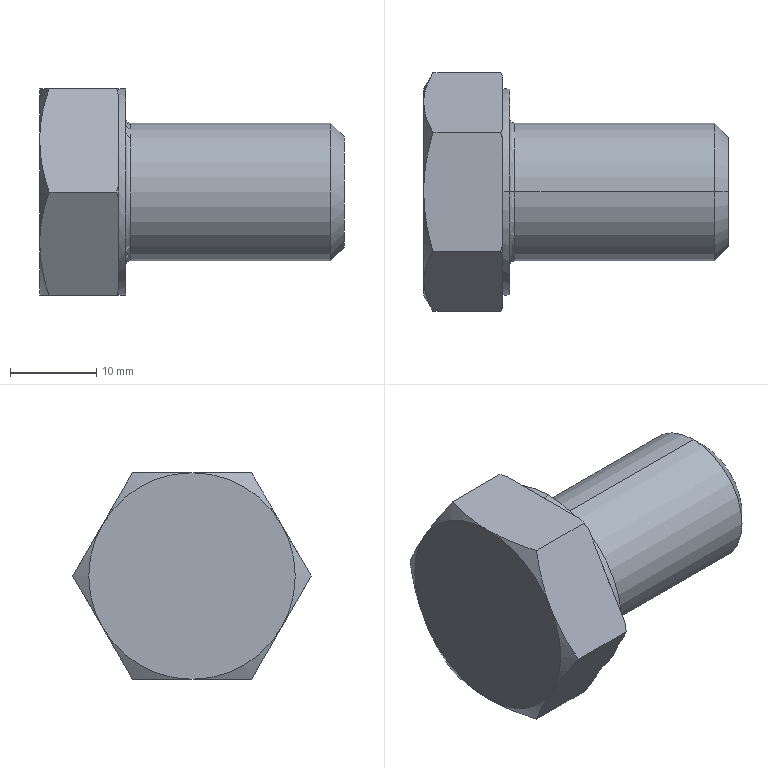Part | SolidWorks | features RevCut 4, Chamfer 1, Extrusion 1, Fillet 1, LPattern 1, Revolution 1 | 1 solid | 35 faces | box 35.4 x 27.713 x 24 mm | volume 9987 mm3 | plane 15 | cone 14 | cylinder 4 | torus 2 | commonest cylinder face diameters 16 x2 24 x2
STEP:
#1=CARTESIAN_POINT('',(10.6,0.,8.));
#2=VERTEX_POINT('',#1);
#3=CARTESIAN_POINT('',(10.6,0.,-8.));
#4=VERTEX_POINT('',#3);
#5=CARTESIAN_POINT('',(10.6,0.,0.));
#6=DIRECTION('',(1.,0.,0.));
#7=DIRECTION('',(0.,0.,-1.));
#8=AXIS2_PLACEMENT_3D('',#5,#6,#7);
#9=CIRCLE('',#8,8.);
#10=EDGE_CURVE('',#2,#4,#9,.T.);
#11=ORIENTED_EDGE('',*,*,#10,.F.);
#12=CARTESIAN_POINT('',(10.,0.,8.6));
#13=VERTEX_POINT('',#12);
#14=CARTESIAN_POINT('',(10.6,0.,8.6));
#15=DIRECTION('',(0.,1.,0.));
#16=DIRECTION('',(0.,0.,1.));
#17=AXIS2_PLACEMENT_3D('',#14,#15,#16);
#18=CIRCLE('',#17,0.6);
#19=EDGE_CURVE('',#2,#13,#18,.T.);
#20=ORIENTED_EDGE('',*,*,#19,.T.);
#21=CARTESIAN_POINT('',(10.,0.,-8.6));
#22=VERTEX_POINT('',#21);
#23=CARTESIAN_POINT('',(10.,0.,0.));
#24=DIRECTION('',(-1.,0.,0.));
#25=DIRECTION('',(0.,0.,-1.));
#26=AXIS2_PLACEMENT_3D('',#23,#24,#25);
#27=CIRCLE('',#26,8.6);
#28=EDGE_CURVE('',#22,#13,#27,.T.);
#29=ORIENTED_EDGE('',*,*,#28,.F.);
#30=CARTESIAN_POINT('',(10.6,0.,-8.6));
#31=DIRECTION('',(0.,-1.,0.));
#32=DIRECTION('',(0.,0.,-1.));
#33=AXIS2_PLACEMENT_3D('',#30,#31,#32);
#34=CIRCLE('',#33,0.6);
#35=EDGE_CURVE('',#4,#22,#34,.T.);
#36=ORIENTED_EDGE('',*,*,#35,.F.);
#37=EDGE_LOOP('',(#11,#20,#29,#36));
#38=FACE_OUTER_BOUND('',#37,.T.);
#39=CARTESIAN_POINT('',(10.6,0.,0.));
#40=DIRECTION('',(1.,0.,0.));
#41=DIRECTION('',(0.,0.,-1.));
#42=AXIS2_PLACEMENT_3D('',#39,#40,#41);
#43=TOROIDAL_SURFACE('',#42,8.6,0.6);
#44=ADVANCED_FACE('',(#38),#43,.F.);
#45=CARTESIAN_POINT('',(35.4,0.,-6.4));
#46=VERTEX_POINT('',#45);
#47=CARTESIAN_POINT('',(35.4,0.,6.4));
#48=VERTEX_POINT('',#47);
#49=CARTESIAN_POINT('',(35.4,0.,0.));
#50=DIRECTION('',(1.,0.,0.));
#51=DIRECTION('',(0.,0.,1.));
#52=AXIS2_PLACEMENT_3D('',#49,#50,#51);
#53=CIRCLE('',#52,6.4);
#54=EDGE_CURVE('',#46,#48,#53,.T.);
#55=ORIENTED_EDGE('',*,*,#54,.F.);
#56=CARTESIAN_POINT('',(33.8,0.,-8.));
#57=VERTEX_POINT('',#56);
#58=CARTESIAN_POINT('',(33.8,0.,-8.));
#59=DIRECTION('',(-0.7071,0.,-0.7071));
#60=VECTOR('',#59,1000.);
#61=LINE('',#58,#60);
#62=EDGE_CURVE('',#46,#57,#61,.T.);
#63=ORIENTED_EDGE('',*,*,#62,.T.);
#64=CARTESIAN_POINT('',(33.8,0.,8.));
#65=VERTEX_POINT('',#64);
#66=CARTESIAN_POINT('',(33.8,0.,0.));
#67=DIRECTION('',(-1.,0.,0.));
#68=DIRECTION('',(0.,0.,1.));
#69=AXIS2_PLACEMENT_3D('',#66,#67,#68);
#70=CIRCLE('',#69,8.);
#71=EDGE_CURVE('',#65,#57,#70,.T.);
#72=ORIENTED_EDGE('',*,*,#71,.F.);
#73=CARTESIAN_POINT('',(33.8,0.,8.));
#74=DIRECTION('',(-0.7071,0.,0.7071));
#75=VECTOR('',#74,1000.);
#76=LINE('',#73,#75);
#77=EDGE_CURVE('',#48,#65,#76,.T.);
#78=ORIENTED_EDGE('',*,*,#77,.F.);
#79=EDGE_LOOP('',(#55,#63,#72,#78));
#80=FACE_OUTER_BOUND('',#79,.T.);
#81=CARTESIAN_POINT('',(33.8,0.,0.));
#82=DIRECTION('',(-1.,0.,0.));
#83=DIRECTION('',(0.,0.,1.));
#84=AXIS2_PLACEMENT_3D('',#81,#82,#83);
#85=CONICAL_SURFACE('',#84,8.,0.7854);
#86=ADVANCED_FACE('',(#80),#85,.T.);
#87=ORIENTED_EDGE('',*,*,#71,.T.);
#88=CARTESIAN_POINT('',(0.,0.,-8.));
#89=DIRECTION('',(-1.,0.,0.));
#90=VECTOR('',#89,1000.);
#91=LINE('',#88,#90);
#92=EDGE_CURVE('',#57,#4,#91,.T.);
#93=ORIENTED_EDGE('',*,*,#92,.T.);
#94=CARTESIAN_POINT('',(10.6,0.,0.));
#95=DIRECTION('',(1.,0.,0.));
#96=DIRECTION('',(0.,0.,-1.));
#97=AXIS2_PLACEMENT_3D('',#94,#95,#96);
#98=CIRCLE('',#97,8.);
#99=EDGE_CURVE('',#4,#2,#98,.T.);
#100=ORIENTED_EDGE('',*,*,#99,.T.);
#101=CARTESIAN_POINT('',(0.,0.,8.));
#102=DIRECTION('',(-1.,0.,0.));
#103=VECTOR('',#102,1000.);
#104=LINE('',#101,#103);
#105=EDGE_CURVE('',#65,#2,#104,.T.);
#106=ORIENTED_EDGE('',*,*,#105,.F.);
#107=EDGE_LOOP('',(#87,#93,#100,#106));
#108=FACE_OUTER_BOUND('',#107,.T.);
#109=CARTESIAN_POINT('',(0.,0.,0.));
#110=DIRECTION('',(-1.,0.,0.));
#111=DIRECTION('',(0.,0.,1.));
#112=AXIS2_PLACEMENT_3D('',#109,#110,#111);
#113=CYLINDRICAL_SURFACE('',#112,8.);
#114=ADVANCED_FACE('',(#108),#113,.T.);
#115=CARTESIAN_POINT('',(10.,0.,-12.));
#116=VERTEX_POINT('',#115);
#117=CARTESIAN_POINT('',(10.,0.,12.));
#118=VERTEX_POINT('',#117);
#119=CARTESIAN_POINT('',(10.,0.,0.));
#120=DIRECTION('',(1.,0.,0.));
#121=DIRECTION('',(0.,0.,-1.));
#122=AXIS2_PLACEMENT_3D('',#119,#120,#121);
#123=CIRCLE('',#122,12.);
#124=EDGE_CURVE('',#116,#118,#123,.T.);
#125=ORIENTED_EDGE('',*,*,#124,.F.);
#126=CARTESIAN_POINT('',(9.2,0.,-12.));
#127=VERTEX_POINT('',#126);
#128=CARTESIAN_POINT('',(0.,0.,-12.));
#129=DIRECTION('',(-1.,0.,0.));
#130=VECTOR('',#129,1000.);
#131=LINE('',#128,#130);
#132=EDGE_CURVE('',#116,#127,#131,.T.);
#133=ORIENTED_EDGE('',*,*,#132,.T.);
#134=CARTESIAN_POINT('',(9.2,10.392,-6.));
#135=VERTEX_POINT('',#134);
#136=CARTESIAN_POINT('',(9.2,0.,0.));
#137=DIRECTION('',(-1.,0.,0.));
#138=DIRECTION('',(0.,0.,1.));
#139=AXIS2_PLACEMENT_3D('',#136,#137,#138);
#140=CIRCLE('',#139,12.);
#141=EDGE_CURVE('',#135,#127,#140,.T.);
#142=ORIENTED_EDGE('',*,*,#141,.F.);
#143=CARTESIAN_POINT('',(9.2,10.392,6.));
#144=VERTEX_POINT('',#143);
#145=CARTESIAN_POINT('',(9.2,0.,0.));
#146=DIRECTION('',(-1.,0.,0.));
#147=DIRECTION('',(0.,0.,1.));
#148=AXIS2_PLACEMENT_3D('',#145,#146,#147);
#149=CIRCLE('',#148,12.);
#150=EDGE_CURVE('',#144,#135,#149,.T.);
#151=ORIENTED_EDGE('',*,*,#150,.F.);
#152=CARTESIAN_POINT('',(9.2,0.,12.));
#153=VERTEX_POINT('',#152);
#154=CARTESIAN_POINT('',(9.2,0.,0.));
#155=DIRECTION('',(-1.,0.,0.));
#156=DIRECTION('',(0.,0.,1.));
#157=AXIS2_PLACEMENT_3D('',#154,#155,#156);
#158=CIRCLE('',#157,12.);
#159=EDGE_CURVE('',#153,#144,#158,.T.);
#160=ORIENTED_EDGE('',*,*,#159,.F.);
#161=CARTESIAN_POINT('',(0.,0.,12.));
#162=DIRECTION('',(-1.,0.,0.));
#163=VECTOR('',#162,1000.);
#164=LINE('',#161,#163);
#165=EDGE_CURVE('',#118,#153,#164,.T.);
#166=ORIENTED_EDGE('',*,*,#165,.F.);
#167=EDGE_LOOP('',(#125,#133,#142,#151,#160,#166));
#168=FACE_OUTER_BOUND('',#167,.T.);
#169=CARTESIAN_POINT('',(0.,0.,0.));
#170=DIRECTION('',(-1.,0.,0.));
#171=DIRECTION('',(0.,0.,1.));
#172=AXIS2_PLACEMENT_3D('',#169,#170,#171);
#173=CYLINDRICAL_SURFACE('',#172,12.);
#174=ADVANCED_FACE('',(#168),#173,.T.);
#175=CARTESIAN_POINT('',(9.2,7.427,-11.136));
#176=VERTEX_POINT('',#175);
#177=CARTESIAN_POINT('',(9.2,6.928,-12.));
#178=DIRECTION('',(0.,0.5,0.866));
#179=VECTOR('',#178,1000.);
#180=LINE('',#177,#179);
#181=EDGE_CURVE('',#176,#135,#180,.T.);
#182=ORIENTED_EDGE('',*,*,#181,.F.);
#183=CARTESIAN_POINT('',(8.928,6.928,-12.));
#184=VERTEX_POINT('',#183);
#185=CARTESIAN_POINT('',(8.928,6.928,-12.));
#186=CARTESIAN_POINT('',(9.024,7.094,-11.713));
#187=CARTESIAN_POINT('',(9.115,7.26,-11.425));
#188=CARTESIAN_POINT('',(9.2,7.427,-11.136));
#189=B_SPLINE_CURVE_WITH_KNOTS('',3,(#185,#186,#187,#188),.UNSPECIFIED.,.F.,.F.,(4,4),(0.000000238,0.001026),.UNSPECIFIED.);
#190=EDGE_CURVE('',#184,#176,#189,.T.);
#191=ORIENTED_EDGE('',*,*,#190,.F.);
#192=CARTESIAN_POINT('',(1.072,6.928,-12.));
#193=VERTEX_POINT('',#192);
#194=CARTESIAN_POINT('',(10.,6.928,-12.));
#195=DIRECTION('',(-1.,0.,0.));
#196=VECTOR('',#195,1000.);
#197=LINE('',#194,#196);
#198=EDGE_CURVE('',#184,#193,#197,.T.);
#199=ORIENTED_EDGE('',*,*,#198,.T.);
#200=CARTESIAN_POINT('',(0.,10.392,-6.));
#201=VERTEX_POINT('',#200);
#202=CARTESIAN_POINT('',(0.,10.392,-6.));
#203=CARTESIAN_POINT('',(0.,10.098,-6.509));
#204=CARTESIAN_POINT('',(0.02533,9.803,-7.021));
#205=CARTESIAN_POINT('',(0.1234,9.219,-8.033));
#206=CARTESIAN_POINT('',(0.196,8.929,-8.535));
#207=CARTESIAN_POINT('',(0.476,8.063,-10.034));
#208=CARTESIAN_POINT('',(0.7454,7.493,-11.021));
#209=CARTESIAN_POINT('',(1.072,6.928,-12.));
#210=B_SPLINE_CURVE_WITH_KNOTS('',3,(#202,#203,#204,#205,#206,#207,#208,#209),.UNSPECIFIED.,.F.,.F.,(4,2,2,4),(0.00701,0.008756,0.0105,0.01399),.UNSPECIFIED.);
#211=EDGE_CURVE('',#201,#193,#210,.T.);
#212=ORIENTED_EDGE('',*,*,#211,.F.);
#213=CARTESIAN_POINT('',(1.072,13.856,0.));
#214=VERTEX_POINT('',#213);
#215=CARTESIAN_POINT('',(1.072,13.856,0.));
#216=CARTESIAN_POINT('',(0.7446,13.29,-0.9815));
#217=CARTESIAN_POINT('',(0.4751,12.719,-1.97));
#218=CARTESIAN_POINT('',(0.1021,11.565,-3.968));
#219=CARTESIAN_POINT('',(0.,10.982,-4.978));
#220=CARTESIAN_POINT('',(0.,10.392,-6.));
#221=B_SPLINE_CURVE_WITH_KNOTS('',3,(#215,#216,#217,#218,#219,#220),.UNSPECIFIED.,.F.,.F.,(4,2,4),(0.000000238,0.003505,0.00701),.UNSPECIFIED.);
#222=EDGE_CURVE('',#214,#201,#221,.T.);
#223=ORIENTED_EDGE('',*,*,#222,.F.);
#224=CARTESIAN_POINT('',(8.928,13.856,0.));
#225=VERTEX_POINT('',#224);
#226=CARTESIAN_POINT('',(10.,13.856,0.));
#227=DIRECTION('',(-1.,0.,0.));
#228=VECTOR('',#227,1000.);
#229=LINE('',#226,#228);
#230=EDGE_CURVE('',#225,#214,#229,.T.);
#231=ORIENTED_EDGE('',*,*,#230,.F.);
#232=CARTESIAN_POINT('',(9.2,13.358,-0.8637));
#233=VERTEX_POINT('',#232);
#234=CARTESIAN_POINT('',(9.2,13.358,-0.8637));
#235=CARTESIAN_POINT('',(9.115,13.524,-0.575));
#236=CARTESIAN_POINT('',(9.024,13.691,-0.2872));
#237=CARTESIAN_POINT('',(8.928,13.856,0.));
#238=B_SPLINE_CURVE_WITH_KNOTS('',3,(#234,#235,#236,#237),.UNSPECIFIED.,.F.,.F.,(4,4),(0.01297,0.01399),.UNSPECIFIED.);
#239=EDGE_CURVE('',#233,#225,#238,.T.);
#240=ORIENTED_EDGE('',*,*,#239,.F.);
#241=CARTESIAN_POINT('',(9.2,6.928,-12.));
#242=DIRECTION('',(0.,0.5,0.866));
#243=VECTOR('',#242,1000.);
#244=LINE('',#241,#243);
#245=EDGE_CURVE('',#135,#233,#244,.T.);
#246=ORIENTED_EDGE('',*,*,#245,.F.);
#247=EDGE_LOOP('',(#182,#191,#199,#212,#223,#231,#240,#246));
#248=FACE_OUTER_BOUND('',#247,.T.);
#249=CARTESIAN_POINT('',(10.,6.928,-12.));
#250=DIRECTION('',(0.,-0.866,0.5));
#251=DIRECTION('',(0.,-0.5,-0.866));
#252=AXIS2_PLACEMENT_3D('',#249,#250,#251);
#253=PLANE('',#252);
#254=ADVANCED_FACE('',(#248),#253,.F.);
#255=CARTESIAN_POINT('',(9.2,13.358,0.8637));
#256=VERTEX_POINT('',#255);
#257=CARTESIAN_POINT('',(9.2,13.856,0.));
#258=DIRECTION('',(0.,-0.5,0.866));
#259=VECTOR('',#258,1000.);
#260=LINE('',#257,#259);
#261=EDGE_CURVE('',#256,#144,#260,.T.);
#262=ORIENTED_EDGE('',*,*,#261,.F.);
#263=CARTESIAN_POINT('',(8.928,13.856,0.));
#264=CARTESIAN_POINT('',(9.024,13.691,0.2873));
#265=CARTESIAN_POINT('',(9.115,13.524,0.5751));
#266=CARTESIAN_POINT('',(9.2,13.358,0.8637));
#267=B_SPLINE_CURVE_WITH_KNOTS('',3,(#263,#264,#265,#266),.UNSPECIFIED.,.F.,.F.,(4,4),(0.000000238,0.001026),.UNSPECIFIED.);
#268=EDGE_CURVE('',#225,#256,#267,.T.);
#269=ORIENTED_EDGE('',*,*,#268,.F.);
#270=ORIENTED_EDGE('',*,*,#230,.T.);
#271=CARTESIAN_POINT('',(0.,10.392,6.));
#272=VERTEX_POINT('',#271);
#273=CARTESIAN_POINT('',(0.,10.392,6.));
#274=CARTESIAN_POINT('',(0.,10.686,5.491));
#275=CARTESIAN_POINT('',(0.02533,10.982,4.979));
#276=CARTESIAN_POINT('',(0.1234,11.566,3.967));
#277=CARTESIAN_POINT('',(0.196,11.856,3.465));
#278=CARTESIAN_POINT('',(0.476,12.721,1.966));
#279=CARTESIAN_POINT('',(0.7454,13.291,0.9791));
#280=CARTESIAN_POINT('',(1.072,13.856,0.));
#281=B_SPLINE_CURVE_WITH_KNOTS('',3,(#273,#274,#275,#276,#277,#278,#279,#280),.UNSPECIFIED.,.F.,.F.,(4,2,2,4),(0.00701,0.008756,0.0105,0.01399),.UNSPECIFIED.);
#282=EDGE_CURVE('',#272,#214,#281,.T.);
#283=ORIENTED_EDGE('',*,*,#282,.F.);
#284=CARTESIAN_POINT('',(1.072,6.928,12.));
#285=VERTEX_POINT('',#284);
#286=CARTESIAN_POINT('',(1.072,6.928,12.));
#287=CARTESIAN_POINT('',(0.7446,7.495,11.018));
#288=CARTESIAN_POINT('',(0.4751,8.066,10.03));
#289=CARTESIAN_POINT('',(0.1021,9.219,8.032));
#290=CARTESIAN_POINT('',(0.,9.802,7.022));
#291=CARTESIAN_POINT('',(0.,10.392,6.));
#292=B_SPLINE_CURVE_WITH_KNOTS('',3,(#286,#287,#288,#289,#290,#291),.UNSPECIFIED.,.F.,.F.,(4,2,4),(0.000000238,0.003505,0.00701),.UNSPECIFIED.);
#293=EDGE_CURVE('',#285,#272,#292,.T.);
#294=ORIENTED_EDGE('',*,*,#293,.F.);
#295=CARTESIAN_POINT('',(8.928,6.928,12.));
#296=VERTEX_POINT('',#295);
#297=CARTESIAN_POINT('',(10.,6.928,12.));
#298=DIRECTION('',(-1.,0.,0.));
#299=VECTOR('',#298,1000.);
#300=LINE('',#297,#299);
#301=EDGE_CURVE('',#296,#285,#300,.T.);
#302=ORIENTED_EDGE('',*,*,#301,.F.);
#303=CARTESIAN_POINT('',(9.2,7.427,11.136));
#304=VERTEX_POINT('',#303);
#305=CARTESIAN_POINT('',(9.2,7.427,11.136));
#306=CARTESIAN_POINT('',(9.115,7.26,11.425));
#307=CARTESIAN_POINT('',(9.024,7.094,11.713));
#308=CARTESIAN_POINT('',(8.928,6.928,12.));
#309=B_SPLINE_CURVE_WITH_KNOTS('',3,(#305,#306,#307,#308),.UNSPECIFIED.,.F.,.F.,(4,4),(0.01297,0.01399),.UNSPECIFIED.);
#310=EDGE_CURVE('',#304,#296,#309,.T.);
#311=ORIENTED_EDGE('',*,*,#310,.F.);
#312=CARTESIAN_POINT('',(9.2,13.856,0.));
#313=DIRECTION('',(0.,-0.5,0.866));
#314=VECTOR('',#313,1000.);
#315=LINE('',#312,#314);
#316=EDGE_CURVE('',#144,#304,#315,.T.);
#317=ORIENTED_EDGE('',*,*,#316,.F.);
#318=EDGE_LOOP('',(#262,#269,#270,#283,#294,#302,#311,#317));
#319=FACE_OUTER_BOUND('',#318,.T.);
#320=CARTESIAN_POINT('',(10.,13.856,0.));
#321=DIRECTION('',(0.,-0.866,-0.5));
#322=DIRECTION('',(0.,0.5,-0.866));
#323=AXIS2_PLACEMENT_3D('',#320,#321,#322);
#324=PLANE('',#323);
#325=ADVANCED_FACE('',(#319),#324,.F.);
#326=CARTESIAN_POINT('',(9.2,5.931,12.));
#327=VERTEX_POINT('',#326);
#328=CARTESIAN_POINT('',(9.2,6.928,12.));
#329=DIRECTION('',(0.,-1.,0.));
#330=VECTOR('',#329,1000.);
#331=LINE('',#328,#330);
#332=EDGE_CURVE('',#327,#153,#331,.T.);
#333=ORIENTED_EDGE('',*,*,#332,.F.);
#334=CARTESIAN_POINT('',(8.928,6.928,12.));
#335=CARTESIAN_POINT('',(9.024,6.597,12.));
#336=CARTESIAN_POINT('',(9.115,6.265,12.));
#337=CARTESIAN_POINT('',(9.2,5.931,12.));
#338=B_SPLINE_CURVE_WITH_KNOTS('',3,(#334,#335,#336,#337),.UNSPECIFIED.,.F.,.F.,(4,4),(0.03236,0.0334),.UNSPECIFIED.);
#339=EDGE_CURVE('',#296,#327,#338,.T.);
#340=ORIENTED_EDGE('',*,*,#339,.F.);
#341=ORIENTED_EDGE('',*,*,#301,.T.);
#342=CARTESIAN_POINT('',(0.,0.,12.));
#343=VERTEX_POINT('',#342);
#344=CARTESIAN_POINT('',(0.,0.,12.));
#345=CARTESIAN_POINT('',(0.,0.5865,12.));
#346=CARTESIAN_POINT('',(0.02506,1.176,12.));
#347=CARTESIAN_POINT('',(0.1242,2.355,12.));
#348=CARTESIAN_POINT('',(0.1975,2.939,12.));
#349=CARTESIAN_POINT('',(0.4791,4.673,12.));
#350=CARTESIAN_POINT('',(0.7483,5.808,12.));
#351=CARTESIAN_POINT('',(1.072,6.928,12.));
#352=B_SPLINE_CURVE_WITH_KNOTS('',3,(#344,#345,#346,#347,#348,#349,#350,#351),.UNSPECIFIED.,.F.,.F.,(4,2,2,4),(0.01982,0.02158,0.02333,0.02684),.UNSPECIFIED.);
#353=EDGE_CURVE('',#343,#285,#352,.T.);
#354=ORIENTED_EDGE('',*,*,#353,.F.);
#355=CARTESIAN_POINT('',(1.072,-6.928,12.));
#356=VERTEX_POINT('',#355);
#357=CARTESIAN_POINT('',(1.072,-6.928,12.));
#358=CARTESIAN_POINT('',(0.7461,-5.8,12.));
#359=CARTESIAN_POINT('',(0.4736,-4.647,12.));
#360=CARTESIAN_POINT('',(0.1008,-2.335,12.));
#361=CARTESIAN_POINT('',(0.,-1.172,12.));
#362=CARTESIAN_POINT('',(0.,0.,12.));
#363=B_SPLINE_CURVE_WITH_KNOTS('',3,(#357,#358,#359,#360,#361,#362),.UNSPECIFIED.,.F.,.F.,(4,2,4),(0.01281,0.01632,0.01982),.UNSPECIFIED.);
#364=EDGE_CURVE('',#356,#343,#363,.T.);
#365=ORIENTED_EDGE('',*,*,#364,.F.);
#366=CARTESIAN_POINT('',(8.928,-6.928,12.));
#367=VERTEX_POINT('',#366);
#368=CARTESIAN_POINT('',(10.,-6.928,12.));
#369=DIRECTION('',(-1.,0.,0.));
#370=VECTOR('',#369,1000.);
#371=LINE('',#368,#370);
#372=EDGE_CURVE('',#367,#356,#371,.T.);
#373=ORIENTED_EDGE('',*,*,#372,.F.);
#374=CARTESIAN_POINT('',(9.2,-5.931,12.));
#375=VERTEX_POINT('',#374);
#376=CARTESIAN_POINT('',(9.2,-5.931,12.));
#377=CARTESIAN_POINT('',(9.114,-6.265,12.));
#378=CARTESIAN_POINT('',(9.024,-6.598,12.));
#379=CARTESIAN_POINT('',(8.928,-6.928,12.));
#380=B_SPLINE_CURVE_WITH_KNOTS('',3,(#376,#377,#378,#379),.UNSPECIFIED.,.F.,.F.,(4,4),(0.04537,0.0464),.UNSPECIFIED.);
#381=EDGE_CURVE('',#375,#367,#380,.T.);
#382=ORIENTED_EDGE('',*,*,#381,.F.);
#383=CARTESIAN_POINT('',(9.2,6.928,12.));
#384=DIRECTION('',(0.,-1.,0.));
#385=VECTOR('',#384,1000.);
#386=LINE('',#383,#385);
#387=EDGE_CURVE('',#153,#375,#386,.T.);
#388=ORIENTED_EDGE('',*,*,#387,.F.);
#389=EDGE_LOOP('',(#333,#340,#341,#354,#365,#373,#382,#388));
#390=FACE_OUTER_BOUND('',#389,.T.);
#391=CARTESIAN_POINT('',(10.,6.928,12.));
#392=DIRECTION('',(0.,0.,-1.));
#393=DIRECTION('',(-1.,0.,0.));
#394=AXIS2_PLACEMENT_3D('',#391,#392,#393);
#395=PLANE('',#394);
#396=ADVANCED_FACE('',(#390),#395,.F.);
#397=CARTESIAN_POINT('',(9.2,-7.427,11.136));
#398=VERTEX_POINT('',#397);
#399=CARTESIAN_POINT('',(9.2,-10.392,6.));
#400=VERTEX_POINT('',#399);
#401=CARTESIAN_POINT('',(9.2,-13.856,0.));
#402=DIRECTION('',(0.,-0.5,-0.866));
#403=VECTOR('',#402,1000.);
#404=LINE('',#401,#403);
#405=EDGE_CURVE('',#398,#400,#404,.T.);
#406=ORIENTED_EDGE('',*,*,#405,.F.);
#407=CARTESIAN_POINT('',(8.928,-6.928,12.));
#408=CARTESIAN_POINT('',(9.024,-7.094,11.713));
#409=CARTESIAN_POINT('',(9.115,-7.26,11.425));
#410=CARTESIAN_POINT('',(9.2,-7.427,11.136));
#411=B_SPLINE_CURVE_WITH_KNOTS('',3,(#407,#408,#409,#410),.UNSPECIFIED.,.F.,.F.,(4,4),(0.000000238,0.001026),.UNSPECIFIED.);
#412=EDGE_CURVE('',#367,#398,#411,.T.);
#413=ORIENTED_EDGE('',*,*,#412,.F.);
#414=ORIENTED_EDGE('',*,*,#372,.T.);
#415=CARTESIAN_POINT('',(0.,-10.392,6.));
#416=VERTEX_POINT('',#415);
#417=CARTESIAN_POINT('',(0.,-10.392,6.));
#418=CARTESIAN_POINT('',(0.,-10.098,6.509));
#419=CARTESIAN_POINT('',(0.02533,-9.803,7.021));
#420=CARTESIAN_POINT('',(0.1234,-9.219,8.033));
#421=CARTESIAN_POINT('',(0.196,-8.929,8.535));
#422=CARTESIAN_POINT('',(0.476,-8.063,10.034));
#423=CARTESIAN_POINT('',(0.7454,-7.493,11.021));
#424=CARTESIAN_POINT('',(1.072,-6.928,12.));
#425=B_SPLINE_CURVE_WITH_KNOTS('',3,(#417,#418,#419,#420,#421,#422,#423,#424),.UNSPECIFIED.,.F.,.F.,(4,2,2,4),(0.00701,0.008756,0.0105,0.01399),.UNSPECIFIED.);
#426=EDGE_CURVE('',#416,#356,#425,.T.);
#427=ORIENTED_EDGE('',*,*,#426,.F.);
#428=CARTESIAN_POINT('',(1.072,-13.856,0.));
#429=VERTEX_POINT('',#428);
#430=CARTESIAN_POINT('',(1.072,-13.856,0.));
#431=CARTESIAN_POINT('',(0.7446,-13.29,0.9815));
#432=CARTESIAN_POINT('',(0.4751,-12.719,1.97));
#433=CARTESIAN_POINT('',(0.1021,-11.565,3.968));
#434=CARTESIAN_POINT('',(0.,-10.982,4.978));
#435=CARTESIAN_POINT('',(0.,-10.392,6.));
#436=B_SPLINE_CURVE_WITH_KNOTS('',3,(#430,#431,#432,#433,#434,#435),.UNSPECIFIED.,.F.,.F.,(4,2,4),(0.000000238,0.003505,0.00701),.UNSPECIFIED.);
#437=EDGE_CURVE('',#429,#416,#436,.T.);
#438=ORIENTED_EDGE('',*,*,#437,.F.);
#439=CARTESIAN_POINT('',(8.928,-13.856,0.));
#440=VERTEX_POINT('',#439);
#441=CARTESIAN_POINT('',(10.,-13.856,0.));
#442=DIRECTION('',(-1.,0.,0.));
#443=VECTOR('',#442,1000.);
#444=LINE('',#441,#443);
#445=EDGE_CURVE('',#440,#429,#444,.T.);
#446=ORIENTED_EDGE('',*,*,#445,.F.);
#447=CARTESIAN_POINT('',(9.2,-13.358,0.8637));
#448=VERTEX_POINT('',#447);
#449=CARTESIAN_POINT('',(9.2,-13.358,0.8637));
#450=CARTESIAN_POINT('',(9.115,-13.524,0.575));
#451=CARTESIAN_POINT('',(9.024,-13.691,0.2872));
#452=CARTESIAN_POINT('',(8.928,-13.856,0.));
#453=B_SPLINE_CURVE_WITH_KNOTS('',3,(#449,#450,#451,#452),.UNSPECIFIED.,.F.,.F.,(4,4),(0.01297,0.01399),.UNSPECIFIED.);
#454=EDGE_CURVE('',#448,#440,#453,.T.);
#455=ORIENTED_EDGE('',*,*,#454,.F.);
#456=CARTESIAN_POINT('',(9.2,-13.856,0.));
#457=DIRECTION('',(0.,-0.5,-0.866));
#458=VECTOR('',#457,1000.);
#459=LINE('',#456,#458);
#460=EDGE_CURVE('',#400,#448,#459,.T.);
#461=ORIENTED_EDGE('',*,*,#460,.F.);
#462=EDGE_LOOP('',(#406,#413,#414,#427,#438,#446,#455,#461));
#463=FACE_OUTER_BOUND('',#462,.T.);
#464=CARTESIAN_POINT('',(10.,-13.856,0.));
#465=DIRECTION('',(0.,0.866,-0.5));
#466=DIRECTION('',(0.,0.5,0.866));
#467=AXIS2_PLACEMENT_3D('',#464,#465,#466);
#468=PLANE('',#467);
#469=ADVANCED_FACE('',(#463),#468,.F.);
#470=CARTESIAN_POINT('',(9.2,-13.358,-0.8637));
#471=VERTEX_POINT('',#470);
#472=CARTESIAN_POINT('',(9.2,-10.392,-6.));
#473=VERTEX_POINT('',#472);
#474=CARTESIAN_POINT('',(9.2,-6.928,-12.));
#475=DIRECTION('',(0.,0.5,-0.866));
#476=VECTOR('',#475,1000.);
#477=LINE('',#474,#476);
#478=EDGE_CURVE('',#471,#473,#477,.T.);
#479=ORIENTED_EDGE('',*,*,#478,.F.);
#480=CARTESIAN_POINT('',(8.928,-13.856,0.));
#481=CARTESIAN_POINT('',(9.024,-13.691,-0.2873));
#482=CARTESIAN_POINT('',(9.115,-13.524,-0.5751));
#483=CARTESIAN_POINT('',(9.2,-13.358,-0.8637));
#484=B_SPLINE_CURVE_WITH_KNOTS('',3,(#480,#481,#482,#483),.UNSPECIFIED.,.F.,.F.,(4,4),(0.000000238,0.001026),.UNSPECIFIED.);
#485=EDGE_CURVE('',#440,#471,#484,.T.);
#486=ORIENTED_EDGE('',*,*,#485,.F.);
#487=ORIENTED_EDGE('',*,*,#445,.T.);
#488=CARTESIAN_POINT('',(0.,-10.392,-6.));
#489=VERTEX_POINT('',#488);
#490=CARTESIAN_POINT('',(0.,-10.392,-6.));
#491=CARTESIAN_POINT('',(0.,-10.686,-5.491));
#492=CARTESIAN_POINT('',(0.02533,-10.982,-4.979));
#493=CARTESIAN_POINT('',(0.1234,-11.566,-3.967));
#494=CARTESIAN_POINT('',(0.196,-11.856,-3.465));
#495=CARTESIAN_POINT('',(0.476,-12.721,-1.966));
#496=CARTESIAN_POINT('',(0.7454,-13.291,-0.9791));
#497=CARTESIAN_POINT('',(1.072,-13.856,0.));
#498=B_SPLINE_CURVE_WITH_KNOTS('',3,(#490,#491,#492,#493,#494,#495,#496,#497),.UNSPECIFIED.,.F.,.F.,(4,2,2,4),(0.00701,0.008756,0.0105,0.01399),.UNSPECIFIED.);
#499=EDGE_CURVE('',#489,#429,#498,.T.);
#500=ORIENTED_EDGE('',*,*,#499,.F.);
#501=CARTESIAN_POINT('',(1.072,-6.928,-12.));
#502=VERTEX_POINT('',#501);
#503=CARTESIAN_POINT('',(1.072,-6.928,-12.));
#504=CARTESIAN_POINT('',(0.7446,-7.495,-11.018));
#505=CARTESIAN_POINT('',(0.4751,-8.066,-10.03));
#506=CARTESIAN_POINT('',(0.1021,-9.219,-8.032));
#507=CARTESIAN_POINT('',(0.,-9.802,-7.022));
#508=CARTESIAN_POINT('',(0.,-10.392,-6.));
#509=B_SPLINE_CURVE_WITH_KNOTS('',3,(#503,#504,#505,#506,#507,#508),.UNSPECIFIED.,.F.,.F.,(4,2,4),(0.000000238,0.003505,0.00701),.UNSPECIFIED.);
#510=EDGE_CURVE('',#502,#489,#509,.T.);
#511=ORIENTED_EDGE('',*,*,#510,.F.);
#512=CARTESIAN_POINT('',(8.928,-6.928,-12.));
#513=VERTEX_POINT('',#512);
#514=CARTESIAN_POINT('',(10.,-6.928,-12.));
#515=DIRECTION('',(-1.,0.,0.));
#516=VECTOR('',#515,1000.);
#517=LINE('',#514,#516);
#518=EDGE_CURVE('',#513,#502,#517,.T.);
#519=ORIENTED_EDGE('',*,*,#518,.F.);
#520=CARTESIAN_POINT('',(9.2,-7.427,-11.136));
#521=VERTEX_POINT('',#520);
#522=CARTESIAN_POINT('',(9.2,-7.427,-11.136));
#523=CARTESIAN_POINT('',(9.115,-7.26,-11.425));
#524=CARTESIAN_POINT('',(9.024,-7.094,-11.713));
#525=CARTESIAN_POINT('',(8.928,-6.928,-12.));
#526=B_SPLINE_CURVE_WITH_KNOTS('',3,(#522,#523,#524,#525),.UNSPECIFIED.,.F.,.F.,(4,4),(0.01297,0.01399),.UNSPECIFIED.);
#527=EDGE_CURVE('',#521,#513,#526,.T.);
#528=ORIENTED_EDGE('',*,*,#527,.F.);
#529=CARTESIAN_POINT('',(9.2,-6.928,-12.));
#530=DIRECTION('',(0.,0.5,-0.866));
#531=VECTOR('',#530,1000.);
#532=LINE('',#529,#531);
#533=EDGE_CURVE('',#473,#521,#532,.T.);
#534=ORIENTED_EDGE('',*,*,#533,.F.);
#535=EDGE_LOOP('',(#479,#486,#487,#500,#511,#519,#528,#534));
#536=FACE_OUTER_BOUND('',#535,.T.);
#537=CARTESIAN_POINT('',(10.,-6.928,-12.));
#538=DIRECTION('',(0.,0.866,0.5));
#539=DIRECTION('',(0.,-0.5,0.866));
#540=AXIS2_PLACEMENT_3D('',#537,#538,#539);
#541=PLANE('',#540);
#542=ADVANCED_FACE('',(#536),#541,.F.);
#543=CARTESIAN_POINT('',(9.2,-5.931,-12.));
#544=VERTEX_POINT('',#543);
#545=CARTESIAN_POINT('',(9.2,6.928,-12.));
#546=DIRECTION('',(0.,1.,0.));
#547=VECTOR('',#546,1000.);
#548=LINE('',#545,#547);
#549=EDGE_CURVE('',#544,#127,#548,.T.);
#550=ORIENTED_EDGE('',*,*,#549,.F.);
#551=CARTESIAN_POINT('',(8.928,-6.928,-12.));
#552=CARTESIAN_POINT('',(9.024,-6.598,-12.));
#553=CARTESIAN_POINT('',(9.114,-6.265,-12.));
#554=CARTESIAN_POINT('',(9.2,-5.931,-12.));
#555=B_SPLINE_CURVE_WITH_KNOTS('',3,(#551,#552,#553,#554),.UNSPECIFIED.,.F.,.F.,(4,4),(0.01281,0.01384),.UNSPECIFIED.);
#556=EDGE_CURVE('',#513,#544,#555,.T.);
#557=ORIENTED_EDGE('',*,*,#556,.F.);
#558=ORIENTED_EDGE('',*,*,#518,.T.);
#559=CARTESIAN_POINT('',(0.,0.,-12.));
#560=VERTEX_POINT('',#559);
#561=CARTESIAN_POINT('',(0.,0.,-12.));
#562=CARTESIAN_POINT('',(0.,-1.172,-12.));
#563=CARTESIAN_POINT('',(0.1008,-2.335,-12.));
#564=CARTESIAN_POINT('',(0.4736,-4.647,-12.));
#565=CARTESIAN_POINT('',(0.7461,-5.8,-12.));
#566=CARTESIAN_POINT('',(1.072,-6.928,-12.));
#567=B_SPLINE_CURVE_WITH_KNOTS('',3,(#561,#562,#563,#564,#565,#566),.UNSPECIFIED.,.F.,.F.,(4,2,4),(0.03938,0.04289,0.0464),.UNSPECIFIED.);
#568=EDGE_CURVE('',#560,#502,#567,.T.);
#569=ORIENTED_EDGE('',*,*,#568,.F.);
#570=CARTESIAN_POINT('',(1.072,6.928,-12.));
#571=CARTESIAN_POINT('',(0.7483,5.808,-12.));
#572=CARTESIAN_POINT('',(0.4791,4.673,-12.));
#573=CARTESIAN_POINT('',(0.1975,2.939,-12.));
#574=CARTESIAN_POINT('',(0.1242,2.355,-12.));
#575=CARTESIAN_POINT('',(0.02506,1.176,-12.));
#576=CARTESIAN_POINT('',(0.,0.5865,-12.));
#577=CARTESIAN_POINT('',(0.,0.,-12.));
#578=B_SPLINE_CURVE_WITH_KNOTS('',3,(#570,#571,#572,#573,#574,#575,#576,#577),.UNSPECIFIED.,.F.,.F.,(4,2,2,4),(0.03236,0.03587,0.03763,0.03938),.UNSPECIFIED.);
#579=EDGE_CURVE('',#193,#560,#578,.T.);
#580=ORIENTED_EDGE('',*,*,#579,.F.);
#581=ORIENTED_EDGE('',*,*,#198,.F.);
#582=CARTESIAN_POINT('',(9.2,5.931,-12.));
#583=VERTEX_POINT('',#582);
#584=CARTESIAN_POINT('',(9.2,5.931,-12.));
#585=CARTESIAN_POINT('',(9.115,6.265,-12.));
#586=CARTESIAN_POINT('',(9.024,6.597,-12.));
#587=CARTESIAN_POINT('',(8.928,6.928,-12.));
#588=B_SPLINE_CURVE_WITH_KNOTS('',3,(#584,#585,#586,#587),.UNSPECIFIED.,.F.,.F.,(4,4),(0.0258,0.02684),.UNSPECIFIED.);
#589=EDGE_CURVE('',#583,#184,#588,.T.);
#590=ORIENTED_EDGE('',*,*,#589,.F.);
#591=CARTESIAN_POINT('',(9.2,6.928,-12.));
#592=DIRECTION('',(0.,1.,0.));
#593=VECTOR('',#592,1000.);
#594=LINE('',#591,#593);
#595=EDGE_CURVE('',#127,#583,#594,.T.);
#596=ORIENTED_EDGE('',*,*,#595,.F.);
#597=EDGE_LOOP('',(#550,#557,#558,#569,#580,#581,#590,#596));
#598=FACE_OUTER_BOUND('',#597,.T.);
#599=CARTESIAN_POINT('',(10.,6.928,-12.));
#600=DIRECTION('',(0.,0.,1.));
#601=DIRECTION('',(0.,-1.,0.));
#602=AXIS2_PLACEMENT_3D('',#599,#600,#601);
#603=PLANE('',#602);
#604=ADVANCED_FACE('',(#598),#603,.F.);
#605=ORIENTED_EDGE('',*,*,#556,.T.);
#606=CARTESIAN_POINT('',(9.2,0.,0.));
#607=DIRECTION('',(-1.,0.,0.));
#608=DIRECTION('',(0.,0.,-1.));
#609=AXIS2_PLACEMENT_3D('',#606,#607,#608);
#610=CIRCLE('',#609,13.386);
#611=EDGE_CURVE('',#544,#521,#610,.T.);
#612=ORIENTED_EDGE('',*,*,#611,.T.);
#613=ORIENTED_EDGE('',*,*,#527,.T.);
#614=EDGE_LOOP('',(#605,#612,#613));
#615=FACE_OUTER_BOUND('',#614,.T.);
#616=CARTESIAN_POINT('',(6.041,0.,0.));
#617=DIRECTION('',(-1.,0.,0.));
#618=DIRECTION('',(0.,0.,1.));
#619=AXIS2_PLACEMENT_3D('',#616,#617,#618);
#620=CONICAL_SURFACE('',#619,18.856,1.047);
#621=ADVANCED_FACE('',(#615),#620,.T.);
#622=ORIENTED_EDGE('',*,*,#485,.T.);
#623=CARTESIAN_POINT('',(9.2,0.,0.));
#624=DIRECTION('',(-1.,0.,0.));
#625=DIRECTION('',(0.,0.,-1.));
#626=AXIS2_PLACEMENT_3D('',#623,#624,#625);
#627=CIRCLE('',#626,13.386);
#628=EDGE_CURVE('',#471,#448,#627,.T.);
#629=ORIENTED_EDGE('',*,*,#628,.T.);
#630=ORIENTED_EDGE('',*,*,#454,.T.);
#631=EDGE_LOOP('',(#622,#629,#630));
#632=FACE_OUTER_BOUND('',#631,.T.);
#633=CARTESIAN_POINT('',(6.041,0.,0.));
#634=DIRECTION('',(-1.,0.,0.));
#635=DIRECTION('',(0.,0.,1.));
#636=AXIS2_PLACEMENT_3D('',#633,#634,#635);
#637=CONICAL_SURFACE('',#636,18.856,1.047);
#638=ADVANCED_FACE('',(#632),#637,.T.);
#639=ORIENTED_EDGE('',*,*,#412,.T.);
#640=CARTESIAN_POINT('',(9.2,0.,0.));
#641=DIRECTION('',(-1.,0.,0.));
#642=DIRECTION('',(0.,0.,-1.));
#643=AXIS2_PLACEMENT_3D('',#640,#641,#642);
#644=CIRCLE('',#643,13.386);
#645=EDGE_CURVE('',#398,#375,#644,.T.);
#646=ORIENTED_EDGE('',*,*,#645,.T.);
#647=ORIENTED_EDGE('',*,*,#381,.T.);
#648=EDGE_LOOP('',(#639,#646,#647));
#649=FACE_OUTER_BOUND('',#648,.T.);
#650=CARTESIAN_POINT('',(6.041,0.,0.));
#651=DIRECTION('',(-1.,0.,0.));
#652=DIRECTION('',(0.,0.,1.));
#653=AXIS2_PLACEMENT_3D('',#650,#651,#652);
#654=CONICAL_SURFACE('',#653,18.856,1.047);
#655=ADVANCED_FACE('',(#649),#654,.T.);
#656=ORIENTED_EDGE('',*,*,#339,.T.);
#657=CARTESIAN_POINT('',(9.2,0.,0.));
#658=DIRECTION('',(-1.,0.,0.));
#659=DIRECTION('',(0.,0.,-1.));
#660=AXIS2_PLACEMENT_3D('',#657,#658,#659);
#661=CIRCLE('',#660,13.386);
#662=EDGE_CURVE('',#327,#304,#661,.T.);
#663=ORIENTED_EDGE('',*,*,#662,.T.);
#664=ORIENTED_EDGE('',*,*,#310,.T.);
#665=EDGE_LOOP('',(#656,#663,#664));
#666=FACE_OUTER_BOUND('',#665,.T.);
#667=CARTESIAN_POINT('',(6.041,0.,0.));
#668=DIRECTION('',(-1.,0.,0.));
#669=DIRECTION('',(0.,0.,1.));
#670=AXIS2_PLACEMENT_3D('',#667,#668,#669);
#671=CONICAL_SURFACE('',#670,18.856,1.047);
#672=ADVANCED_FACE('',(#666),#671,.T.);
#673=ORIENTED_EDGE('',*,*,#268,.T.);
#674=CARTESIAN_POINT('',(9.2,0.,0.));
#675=DIRECTION('',(-1.,0.,0.));
#676=DIRECTION('',(0.,0.,-1.));
#677=AXIS2_PLACEMENT_3D('',#674,#675,#676);
#678=CIRCLE('',#677,13.386);
#679=EDGE_CURVE('',#256,#233,#678,.T.);
#680=ORIENTED_EDGE('',*,*,#679,.T.);
#681=ORIENTED_EDGE('',*,*,#239,.T.);
#682=EDGE_LOOP('',(#673,#680,#681));
#683=FACE_OUTER_BOUND('',#682,.T.);
#684=CARTESIAN_POINT('',(6.041,0.,0.));
#685=DIRECTION('',(-1.,0.,0.));
#686=DIRECTION('',(0.,0.,1.));
#687=AXIS2_PLACEMENT_3D('',#684,#685,#686);
#688=CONICAL_SURFACE('',#687,18.856,1.047);
#689=ADVANCED_FACE('',(#683),#688,.T.);
#690=ORIENTED_EDGE('',*,*,#190,.T.);
#691=CARTESIAN_POINT('',(9.2,0.,0.));
#692=DIRECTION('',(-1.,0.,0.));
#693=DIRECTION('',(0.,0.,-1.));
#694=AXIS2_PLACEMENT_3D('',#691,#692,#693);
#695=CIRCLE('',#694,13.386);
#696=EDGE_CURVE('',#176,#583,#695,.T.);
#697=ORIENTED_EDGE('',*,*,#696,.T.);
#698=ORIENTED_EDGE('',*,*,#589,.T.);
#699=EDGE_LOOP('',(#690,#697,#698));
#700=FACE_OUTER_BOUND('',#699,.T.);
#701=CARTESIAN_POINT('',(6.041,0.,0.));
#702=DIRECTION('',(-1.,0.,0.));
#703=DIRECTION('',(0.,0.,1.));
#704=AXIS2_PLACEMENT_3D('',#701,#702,#703);
#705=CONICAL_SURFACE('',#704,18.856,1.047);
#706=ADVANCED_FACE('',(#700),#705,.T.);
#707=ORIENTED_EDGE('',*,*,#510,.T.);
#708=CARTESIAN_POINT('',(0.,0.,0.));
#709=DIRECTION('',(1.,0.,0.));
#710=DIRECTION('',(0.,0.,-1.));
#711=AXIS2_PLACEMENT_3D('',#708,#709,#710);
#712=CIRCLE('',#711,12.);
#713=EDGE_CURVE('',#489,#560,#712,.T.);
#714=ORIENTED_EDGE('',*,*,#713,.T.);
#715=ORIENTED_EDGE('',*,*,#568,.T.);
#716=EDGE_LOOP('',(#707,#714,#715));
#717=FACE_OUTER_BOUND('',#716,.T.);
#718=CARTESIAN_POINT('',(0.,0.,0.));
#719=DIRECTION('',(1.,0.,0.));
#720=DIRECTION('',(0.,0.,-1.));
#721=AXIS2_PLACEMENT_3D('',#718,#719,#720);
#722=CONICAL_SURFACE('',#721,12.,1.047);
#723=ADVANCED_FACE('',(#717),#722,.T.);
#724=ORIENTED_EDGE('',*,*,#437,.T.);
#725=CARTESIAN_POINT('',(0.,0.,0.));
#726=DIRECTION('',(1.,0.,0.));
#727=DIRECTION('',(0.,0.,-1.));
#728=AXIS2_PLACEMENT_3D('',#725,#726,#727);
#729=CIRCLE('',#728,12.);
#730=EDGE_CURVE('',#416,#489,#729,.T.);
#731=ORIENTED_EDGE('',*,*,#730,.T.);
#732=ORIENTED_EDGE('',*,*,#499,.T.);
#733=EDGE_LOOP('',(#724,#731,#732));
#734=FACE_OUTER_BOUND('',#733,.T.);
#735=CARTESIAN_POINT('',(0.,0.,0.));
#736=DIRECTION('',(1.,0.,0.));
#737=DIRECTION('',(0.,0.,-1.));
#738=AXIS2_PLACEMENT_3D('',#735,#736,#737);
#739=CONICAL_SURFACE('',#738,12.,1.047);
#740=ADVANCED_FACE('',(#734),#739,.T.);
#741=ORIENTED_EDGE('',*,*,#364,.T.);
#742=CARTESIAN_POINT('',(0.,0.,0.));
#743=DIRECTION('',(1.,0.,0.));
#744=DIRECTION('',(0.,0.,-1.));
#745=AXIS2_PLACEMENT_3D('',#742,#743,#744);
#746=CIRCLE('',#745,12.);
#747=EDGE_CURVE('',#343,#416,#746,.T.);
#748=ORIENTED_EDGE('',*,*,#747,.T.);
#749=ORIENTED_EDGE('',*,*,#426,.T.);
#750=EDGE_LOOP('',(#741,#748,#749));
#751=FACE_OUTER_BOUND('',#750,.T.);
#752=CARTESIAN_POINT('',(0.,0.,0.));
#753=DIRECTION('',(1.,0.,0.));
#754=DIRECTION('',(0.,0.,-1.));
#755=AXIS2_PLACEMENT_3D('',#752,#753,#754);
#756=CONICAL_SURFACE('',#755,12.,1.047);
#757=ADVANCED_FACE('',(#751),#756,.T.);
#758=ORIENTED_EDGE('',*,*,#353,.T.);
#759=ORIENTED_EDGE('',*,*,#293,.T.);
#760=CARTESIAN_POINT('',(0.,0.,0.));
#761=DIRECTION('',(-1.,0.,0.));
#762=DIRECTION('',(0.,0.,1.));
#763=AXIS2_PLACEMENT_3D('',#760,#761,#762);
#764=CIRCLE('',#763,12.);
#765=EDGE_CURVE('',#343,#272,#764,.T.);
#766=ORIENTED_EDGE('',*,*,#765,.F.);
#767=EDGE_LOOP('',(#758,#759,#766));
#768=FACE_OUTER_BOUND('',#767,.T.);
#769=CARTESIAN_POINT('',(0.,0.,0.));
#770=DIRECTION('',(1.,0.,0.));
#771=DIRECTION('',(0.,0.,-1.));
#772=AXIS2_PLACEMENT_3D('',#769,#770,#771);
#773=CONICAL_SURFACE('',#772,12.,1.047);
#774=ADVANCED_FACE('',(#768),#773,.T.);
#775=ORIENTED_EDGE('',*,*,#282,.T.);
#776=ORIENTED_EDGE('',*,*,#222,.T.);
#777=CARTESIAN_POINT('',(0.,0.,0.));
#778=DIRECTION('',(1.,0.,0.));
#779=DIRECTION('',(0.,0.,-1.));
#780=AXIS2_PLACEMENT_3D('',#777,#778,#779);
#781=CIRCLE('',#780,12.);
#782=EDGE_CURVE('',#201,#272,#781,.T.);
#783=ORIENTED_EDGE('',*,*,#782,.T.);
#784=EDGE_LOOP('',(#775,#776,#783));
#785=FACE_OUTER_BOUND('',#784,.T.);
#786=CARTESIAN_POINT('',(0.,0.,0.));
#787=DIRECTION('',(1.,0.,0.));
#788=DIRECTION('',(0.,0.,-1.));
#789=AXIS2_PLACEMENT_3D('',#786,#787,#788);
#790=CONICAL_SURFACE('',#789,12.,1.047);
#791=ADVANCED_FACE('',(#785),#790,.T.);
#792=ORIENTED_EDGE('',*,*,#211,.T.);
#793=ORIENTED_EDGE('',*,*,#579,.T.);
#794=CARTESIAN_POINT('',(0.,0.,0.));
#795=DIRECTION('',(1.,0.,0.));
#796=DIRECTION('',(0.,0.,-1.));
#797=AXIS2_PLACEMENT_3D('',#794,#795,#796);
#798=CIRCLE('',#797,12.);
#799=EDGE_CURVE('',#560,#201,#798,.T.);
#800=ORIENTED_EDGE('',*,*,#799,.T.);
#801=EDGE_LOOP('',(#792,#793,#800));
#802=FACE_OUTER_BOUND('',#801,.T.);
#803=CARTESIAN_POINT('',(0.,0.,0.));
#804=DIRECTION('',(1.,0.,0.));
#805=DIRECTION('',(0.,0.,-1.));
#806=AXIS2_PLACEMENT_3D('',#803,#804,#805);
#807=CONICAL_SURFACE('',#806,12.,1.047);
#808=ADVANCED_FACE('',(#802),#807,.T.);
#809=ORIENTED_EDGE('',*,*,#799,.F.);
#810=ORIENTED_EDGE('',*,*,#713,.F.);
#811=ORIENTED_EDGE('',*,*,#730,.F.);
#812=ORIENTED_EDGE('',*,*,#747,.F.);
#813=ORIENTED_EDGE('',*,*,#765,.T.);
#814=ORIENTED_EDGE('',*,*,#782,.F.);
#815=EDGE_LOOP('',(#809,#810,#811,#812,#813,#814));
#816=FACE_OUTER_BOUND('',#815,.T.);
#817=CARTESIAN_POINT('',(0.,13.856,0.));
#818=DIRECTION('',(1.,0.,0.));
#819=DIRECTION('',(0.,0.,-1.));
#820=AXIS2_PLACEMENT_3D('',#817,#818,#819);
#821=PLANE('',#820);
#822=ADVANCED_FACE('',(#816),#821,.F.);
#823=ORIENTED_EDGE('',*,*,#387,.T.);
#824=ORIENTED_EDGE('',*,*,#645,.F.);
#825=ORIENTED_EDGE('',*,*,#405,.T.);
#826=CARTESIAN_POINT('',(9.2,0.,0.));
#827=DIRECTION('',(-1.,0.,0.));
#828=DIRECTION('',(0.,0.,1.));
#829=AXIS2_PLACEMENT_3D('',#826,#827,#828);
#830=CIRCLE('',#829,12.);
#831=EDGE_CURVE('',#400,#153,#830,.T.);
#832=ORIENTED_EDGE('',*,*,#831,.T.);
#833=EDGE_LOOP('',(#823,#824,#825,#832));
#834=FACE_OUTER_BOUND('',#833,.T.);
#835=CARTESIAN_POINT('',(9.2,12.,0.));
#836=DIRECTION('',(1.,0.,0.));
#837=DIRECTION('',(0.,0.,-1.));
#838=AXIS2_PLACEMENT_3D('',#835,#836,#837);
#839=PLANE('',#838);
#840=ADVANCED_FACE('',(#834),#839,.T.);
#841=ORIENTED_EDGE('',*,*,#261,.T.);
#842=ORIENTED_EDGE('',*,*,#150,.T.);
#843=ORIENTED_EDGE('',*,*,#245,.T.);
#844=ORIENTED_EDGE('',*,*,#679,.F.);
#845=EDGE_LOOP('',(#841,#842,#843,#844));
#846=FACE_OUTER_BOUND('',#845,.T.);
#847=CARTESIAN_POINT('',(9.2,12.,0.));
#848=DIRECTION('',(1.,0.,0.));
#849=DIRECTION('',(0.,0.,-1.));
#850=AXIS2_PLACEMENT_3D('',#847,#848,#849);
#851=PLANE('',#850);
#852=ADVANCED_FACE('',(#846),#851,.T.);
#853=ORIENTED_EDGE('',*,*,#460,.T.);
#854=ORIENTED_EDGE('',*,*,#628,.F.);
#855=ORIENTED_EDGE('',*,*,#478,.T.);
#856=CARTESIAN_POINT('',(9.2,0.,0.));
#857=DIRECTION('',(-1.,0.,0.));
#858=DIRECTION('',(0.,0.,1.));
#859=AXIS2_PLACEMENT_3D('',#856,#857,#858);
#860=CIRCLE('',#859,12.);
#861=EDGE_CURVE('',#473,#400,#860,.T.);
#862=ORIENTED_EDGE('',*,*,#861,.T.);
#863=EDGE_LOOP('',(#853,#854,#855,#862));
#864=FACE_OUTER_BOUND('',#863,.T.);
#865=CARTESIAN_POINT('',(9.2,12.,0.));
#866=DIRECTION('',(1.,0.,0.));
#867=DIRECTION('',(0.,0.,-1.));
#868=AXIS2_PLACEMENT_3D('',#865,#866,#867);
#869=PLANE('',#868);
#870=ADVANCED_FACE('',(#864),#869,.T.);
#871=ORIENTED_EDGE('',*,*,#533,.T.);
#872=ORIENTED_EDGE('',*,*,#611,.F.);
#873=ORIENTED_EDGE('',*,*,#549,.T.);
#874=CARTESIAN_POINT('',(9.2,0.,0.));
#875=DIRECTION('',(-1.,0.,0.));
#876=DIRECTION('',(0.,0.,1.));
#877=AXIS2_PLACEMENT_3D('',#874,#875,#876);
#878=CIRCLE('',#877,12.);
#879=EDGE_CURVE('',#127,#473,#878,.T.);
#880=ORIENTED_EDGE('',*,*,#879,.T.);
#881=EDGE_LOOP('',(#871,#872,#873,#880));
#882=FACE_OUTER_BOUND('',#881,.T.);
#883=CARTESIAN_POINT('',(9.2,12.,0.));
#884=DIRECTION('',(1.,0.,0.));
#885=DIRECTION('',(0.,0.,-1.));
#886=AXIS2_PLACEMENT_3D('',#883,#884,#885);
#887=PLANE('',#886);
#888=ADVANCED_FACE('',(#882),#887,.T.);
#889=ORIENTED_EDGE('',*,*,#181,.T.);
#890=ORIENTED_EDGE('',*,*,#141,.T.);
#891=ORIENTED_EDGE('',*,*,#595,.T.);
#892=ORIENTED_EDGE('',*,*,#696,.F.);
#893=EDGE_LOOP('',(#889,#890,#891,#892));
#894=FACE_OUTER_BOUND('',#893,.T.);
#895=CARTESIAN_POINT('',(9.2,12.,0.));
#896=DIRECTION('',(1.,0.,0.));
#897=DIRECTION('',(0.,0.,-1.));
#898=AXIS2_PLACEMENT_3D('',#895,#896,#897);
#899=PLANE('',#898);
#900=ADVANCED_FACE('',(#894),#899,.T.);
#901=ORIENTED_EDGE('',*,*,#132,.F.);
#902=CARTESIAN_POINT('',(10.,0.,0.));
#903=DIRECTION('',(1.,0.,0.));
#904=DIRECTION('',(0.,0.,-1.));
#905=AXIS2_PLACEMENT_3D('',#902,#903,#904);
#906=CIRCLE('',#905,12.);
#907=EDGE_CURVE('',#118,#116,#906,.T.);
#908=ORIENTED_EDGE('',*,*,#907,.F.);
#909=ORIENTED_EDGE('',*,*,#165,.T.);
#910=ORIENTED_EDGE('',*,*,#831,.F.);
#911=ORIENTED_EDGE('',*,*,#861,.F.);
#912=ORIENTED_EDGE('',*,*,#879,.F.);
#913=EDGE_LOOP('',(#901,#908,#909,#910,#911,#912));
#914=FACE_OUTER_BOUND('',#913,.T.);
#915=CARTESIAN_POINT('',(0.,0.,0.));
#916=DIRECTION('',(-1.,0.,0.));
#917=DIRECTION('',(0.,0.,1.));
#918=AXIS2_PLACEMENT_3D('',#915,#916,#917);
#919=CYLINDRICAL_SURFACE('',#918,12.);
#920=ADVANCED_FACE('',(#914),#919,.T.);
#921=ORIENTED_EDGE('',*,*,#332,.T.);
#922=ORIENTED_EDGE('',*,*,#159,.T.);
#923=ORIENTED_EDGE('',*,*,#316,.T.);
#924=ORIENTED_EDGE('',*,*,#662,.F.);
#925=EDGE_LOOP('',(#921,#922,#923,#924));
#926=FACE_OUTER_BOUND('',#925,.T.);
#927=CARTESIAN_POINT('',(9.2,12.,0.));
#928=DIRECTION('',(1.,0.,0.));
#929=DIRECTION('',(0.,0.,-1.));
#930=AXIS2_PLACEMENT_3D('',#927,#928,#929);
#931=PLANE('',#930);
#932=ADVANCED_FACE('',(#926),#931,.T.);
#933=CARTESIAN_POINT('',(35.4,0.,0.));
#934=DIRECTION('',(1.,0.,0.));
#935=DIRECTION('',(0.,0.,1.));
#936=AXIS2_PLACEMENT_3D('',#933,#934,#935);
#937=CIRCLE('',#936,6.4);
#938=EDGE_CURVE('',#48,#46,#937,.T.);
#939=ORIENTED_EDGE('',*,*,#938,.T.);
#940=ORIENTED_EDGE('',*,*,#54,.T.);
#941=EDGE_LOOP('',(#939,#940));
#942=FACE_OUTER_BOUND('',#941,.T.);
#943=CARTESIAN_POINT('',(35.4,0.,0.));
#944=DIRECTION('',(-1.,0.,0.));
#945=DIRECTION('',(0.,0.,1.));
#946=AXIS2_PLACEMENT_3D('',#943,#944,#945);
#947=PLANE('',#946);
#948=ADVANCED_FACE('',(#942),#947,.F.);
#949=ORIENTED_EDGE('',*,*,#92,.F.);
#950=CARTESIAN_POINT('',(33.8,0.,0.));
#951=DIRECTION('',(-1.,0.,0.));
#952=DIRECTION('',(0.,0.,1.));
#953=AXIS2_PLACEMENT_3D('',#950,#951,#952);
#954=CIRCLE('',#953,8.);
#955=EDGE_CURVE('',#57,#65,#954,.T.);
#956=ORIENTED_EDGE('',*,*,#955,.T.);
#957=ORIENTED_EDGE('',*,*,#105,.T.);
#958=ORIENTED_EDGE('',*,*,#10,.T.);
#959=EDGE_LOOP('',(#949,#956,#957,#958));
#960=FACE_OUTER_BOUND('',#959,.T.);
#961=CARTESIAN_POINT('',(0.,0.,0.));
#962=DIRECTION('',(-1.,0.,0.));
#963=DIRECTION('',(0.,0.,1.));
#964=AXIS2_PLACEMENT_3D('',#961,#962,#963);
#965=CYLINDRICAL_SURFACE('',#964,8.);
#966=ADVANCED_FACE('',(#960),#965,.T.);
#967=ORIENTED_EDGE('',*,*,#28,.T.);
#968=CARTESIAN_POINT('',(10.,0.,0.));
#969=DIRECTION('',(-1.,0.,0.));
#970=DIRECTION('',(0.,0.,-1.));
#971=AXIS2_PLACEMENT_3D('',#968,#969,#970);
#972=CIRCLE('',#971,8.6);
#973=EDGE_CURVE('',#13,#22,#972,.T.);
#974=ORIENTED_EDGE('',*,*,#973,.T.);
#975=EDGE_LOOP('',(#967,#974));
#976=FACE_BOUND('',#975,.T.);
#977=ORIENTED_EDGE('',*,*,#907,.T.);
#978=ORIENTED_EDGE('',*,*,#124,.T.);
#979=EDGE_LOOP('',(#977,#978));
#980=FACE_OUTER_BOUND('',#979,.T.);
#981=CARTESIAN_POINT('',(10.,13.856,0.));
#982=DIRECTION('',(1.,0.,0.));
#983=DIRECTION('',(0.,0.,-1.));
#984=AXIS2_PLACEMENT_3D('',#981,#982,#983);
#985=PLANE('',#984);
#986=ADVANCED_FACE('',(#976,#980),#985,.T.);
#987=ORIENTED_EDGE('',*,*,#62,.F.);
#988=ORIENTED_EDGE('',*,*,#938,.F.);
#989=ORIENTED_EDGE('',*,*,#77,.T.);
#990=ORIENTED_EDGE('',*,*,#955,.F.);
#991=EDGE_LOOP('',(#987,#988,#989,#990));
#992=FACE_OUTER_BOUND('',#991,.T.);
#993=CARTESIAN_POINT('',(33.8,0.,0.));
#994=DIRECTION('',(-1.,0.,0.));
#995=DIRECTION('',(0.,0.,1.));
#996=AXIS2_PLACEMENT_3D('',#993,#994,#995);
#997=CONICAL_SURFACE('',#996,8.,0.7854);
#998=ADVANCED_FACE('',(#992),#997,.T.);
#999=ORIENTED_EDGE('',*,*,#19,.F.);
#1000=ORIENTED_EDGE('',*,*,#99,.F.);
#1001=ORIENTED_EDGE('',*,*,#35,.T.);
#1002=ORIENTED_EDGE('',*,*,#973,.F.);
#1003=EDGE_LOOP('',(#999,#1000,#1001,#1002));
#1004=FACE_OUTER_BOUND('',#1003,.T.);
#1005=CARTESIAN_POINT('',(10.6,0.,0.));
#1006=DIRECTION('',(1.,0.,0.));
#1007=DIRECTION('',(0.,0.,-1.));
#1008=AXIS2_PLACEMENT_3D('',#1005,#1006,#1007);
#1009=TOROIDAL_SURFACE('',#1008,8.6,0.6);
#1010=ADVANCED_FACE('',(#1004),#1009,.F.);
#1011=CLOSED_SHELL('',(#44,#86,#114,#174,#254,#325,#396,#469,#542,#604,#621,#638,#655,#672,#689,#706,#723,#740,#757,#774,#791,#808,#822,#840,#852,#870,#888,#900,#920,#932,#948,#966,#986,#998,#1010));
#1012=MANIFOLD_SOLID_BREP('',#1011);
#1013=CARTESIAN_POINT('',(0.,0.,0.));
#1014=DIRECTION('',(0.,0.,1.));
#1015=DIRECTION('',(1.,0.,0.));
#1016=AXIS2_PLACEMENT_3D('',#1013,#1014,#1015);
#1017=(LENGTH_UNIT()NAMED_UNIT(*)SI_UNIT(.MILLI.,.METRE.));
#1018=UNCERTAINTY_MEASURE_WITH_UNIT(LENGTH_MEASURE(0.00001),#1017,'','');
#1019=(NAMED_UNIT(*)PLANE_ANGLE_UNIT()SI_UNIT($,.RADIAN.));
#1020=(NAMED_UNIT(*)SI_UNIT($,.STERADIAN.)SOLID_ANGLE_UNIT());
#1021=(GEOMETRIC_REPRESENTATION_CONTEXT(3)GLOBAL_UNCERTAINTY_ASSIGNED_CONTEXT((#1018))GLOBAL_UNIT_ASSIGNED_CONTEXT((#1017,#1019,#1020))REPRESENTATION_CONTEXT('',''));
#1022=ADVANCED_BREP_SHAPE_REPRESENTATION('',(#1012,#1016),#1021);